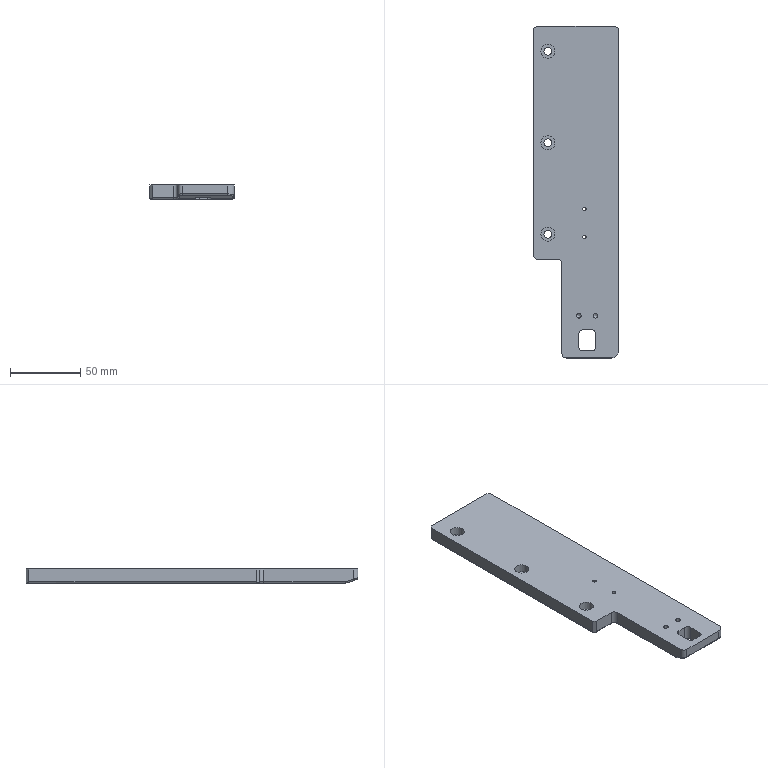NC program | NX | posted with a generic post | part box 60 x 236 x 10 mm
Lines 1 to 1176 of 2922:
N10 G17 G21 G94 G90
(FLOOR_WALL , TOOL : D80)
N12 T19 M6
N14 G54
N16 G17 G0 G90 X281. Y-30. S6500 M3
N18 G43 Z30. H19
N20 Z3.
N22 G94 G1 Z0. F1500.
N24 X278.
N26 X-42.
N28 X-45.
N30 Z3.
N32 G0 Z30.
N34 M5
(DRILLING , TOOL : D6A45)
N36 T01 M6
N38 G54
N40 G17 G0 G90 X18. Y-10. S9500 M3
N42 G43 Z30. H1
N44 G94 G81 G98 Z-1.8 F250. R3.
N46 X83.
N48 X130. Y-36.
N50 X150.
N52 X148. Y-10.
N54 G80
N56 G0 X148. Y-10. Z30.
N58 M5
(DRILLING_COPY_COPY , TOOL : 5.5ZT)
N60 T09 M6
N62 G54
N64 G17 G0 G90 X18. Y-10. S2000 M3
N66 G43 Z30. H9
N68 G94 G83 G98 Z-12.152 F150. Q2. R3.
N70 X83.
N72 X148.
N74 G80
N76 G0 X148. Y-10. Z30.
N78 M5
(DRILLING_COPY_COPY_COPY , TOOL : 2.5ZT)
N80 T02 M6
N82 G54
N84 G17 G0 G90 X130. Y-36. S2000 M3
N86 G43 Z30. H2
N88 G94 G83 G98 Z-11.101 F100. Q2. R3.
N90 X150.
N92 G80
N94 G0 X150. Y-36. Z30.
N96 M5
(ZLEVEL_PROFILE , TOOL : D10)
N98 T15 M6
N100 G54
N102 G17 G0 G90 X163.825 Y9.935 S9500 M3
N104 G43 Z30. H15
N106 Z0.5
N108 G94 G1 Z-1. F1000.
N110 X163.436 Y8.478
N112 G3 X163.695 Y7.512 R1.
N114 G1 X167.606 Y3.606 F3000.
N116 X169.606 Y1.606
N118 G2 X171.1 Y-2. R5.1
N120 G1 Y-14.9
N122 X232.971
N124 G2 X237.356 Y-16.175 R8.333
N126 X240.785 Y-20.779 R7.942
N128 X241.1 Y-23.02 R8.212
N130 G1 Y-54.977
N132 G2 X240.184 Y-59.287 R11.247
N134 X237.644 Y-62.662 R12.774
N136 X234.723 Y-64.384 R11.855
N138 X230.988 Y-65.098 R10.499
N140 G1 X229.803 Y-65.097
N142 X227.433
N144 G3 X226.567 Y-65.597 R1.
N146 G1 X225.701 Y-67.098
N148 Z0.5
N150 G0 X229.287 Y-67.1 Z-0.5
N152 G1 Z-2. F1000.
N154 X230.127 Y-65.608
N156 G2 X230.988 Y-65.099 R1.
N158 G3 X234.765 Y-64.369 R10.736 F3000.
N160 X237.644 Y-62.662 R11.866
N162 X240.184 Y-59.287 R12.774
N164 X241.1 Y-54.977 R11.247
N166 G1 Y-23.02
N168 G3 X240.785 Y-20.779 R8.212
N170 X237.333 Y-16.161 R7.942
N172 X232.971 Y-14.9 R8.333
N174 G1 X171.1
N176 Y-2.
N178 G3 X169.606 Y1.606 R5.1
N180 G1 X167.607 Y3.606
N182 G2 X167.348 Y4.572 R1.
N184 G1 X167.796 Y6.244
N186 Z-0.5
N188 G0 Y6.242 Z-1.5
N190 G1 Z-3. F1000.
N192 X167.348 Y4.572
N194 G3 X167.607 Y3.606 R1.
N196 G1 X169.606 Y1.606 F3000.
N198 G2 X171.1 Y-2. R5.1
N200 G1 Y-14.9
N202 X233.
N204 G2 X241.1 Y-23. R8.1
N206 G1 Y-55.
N208 G2 X238.813 Y-61.401 R10.1
N210 G1 X238.743 Y-61.485
N212 G2 X237.237 Y-62.944 R10.1
N214 G1 X237.12 Y-63.035
N216 G2 X231. Y-65.1 R10.1
N218 G3 X230.134 Y-65.6 R1.
N220 G1 X229.268 Y-67.1
N222 Z-1.5
N224 G0 Z30.
N226 X163.826 Y9.935
N228 Z-0.5
N230 G1 Z-2. F1000.
N232 X163.436 Y8.478
N234 G3 X163.696 Y7.512 R1.
N236 G1 X167.602 Y3.611 F3000.
N238 G3 X168.568 Y3.353 R1.
N240 G1 X170.239 Y3.802
N242 Z-0.5
N244 G0 X167.917 Y6.122 Z-1.5
N246 G1 Z-3. F1000.
N248 X166.694 Y4.898
N250 G2 X167.152 Y4.009 R1.
N252 G1 X167.154 Y4.056 F3000.
N254 X163.696 Y7.512
N256 G2 X163.437 Y8.478 R1.
N258 G1 X163.827 Y9.935
N260 Z-1.5
N262 G0 X163.826 Y9.936 Z-2.5
N264 G1 Z-4. F1000.
N266 X163.437 Y8.478
N268 G3 X163.696 Y7.512 R1.
N270 G1 X167.602 Y3.61 F3000.
N272 G3 X168.568 Y3.352 R1.
N274 G1 X170.24 Y3.801
N276 Z-2.5
N278 G0 Y3.8 Z-3.5
N280 G1 Z-5. F1000.
N282 X168.569 Y3.352
N284 G2 X167.603 Y3.61 R1.
N286 G1 X163.696 Y7.513 F3000.
N288 G2 X163.437 Y8.478 R1.
N290 G1 X163.827 Y9.936
N292 Z-3.5
N294 G0 Z-4.5
N296 G1 Z-6. F1000.
N298 X163.437 Y8.479
N300 G3 X163.696 Y7.513 R1.
N302 G1 X167.603 Y3.61 F3000.
N304 G3 X168.569 Y3.351 R1.
N306 G1 X170.241 Y3.8
N308 Z-4.5
N310 G0 Z-5.5
N312 G1 Z-7. F1000.
N314 X168.569 Y3.351
N316 G2 X167.603 Y3.609 R1.
N318 G1 X163.696 Y7.513 F3000.
N320 G2 X163.437 Y8.479 R1.
N322 G1 X163.827 Y9.936
N324 Z-5.5
N326 G0 Y9.937 Z-6.5
N328 G1 Z-8. F1000.
N330 X163.437 Y8.479
N332 G3 X163.697 Y7.513 R1.
N334 G1 X167.604 Y3.609 F3000.
N336 G3 X168.57 Y3.35 R1.
N338 G1 X170.242 Y3.799
N340 Z-6.5
N342 G0 Z-7.5
N344 G1 Z-9. F1000.
N346 X168.57 Y3.35
N348 G2 X167.604 Y3.609 R1.
N350 G1 X163.697 Y7.513 F3000.
N352 G2 X163.438 Y8.479 R1.
N354 G1 X163.828 Y9.937
N356 Z-7.5
N358 G0 Z-8.5
N360 G1 Z-10. F1000.
N362 X163.438 Y8.479
N364 G3 X163.697 Y7.513 R1.
N366 G1 X167.604 Y3.608 F3000.
N368 G3 X168.57 Y3.35 R1.
N370 G1 X170.243 Y3.798
N372 Z-8.5
N374 G0 Z30.
N376 X167.796 Y6.244
N378 Z-2.5
N380 G1 Z-4. F1000.
N382 X167.348 Y4.572
N384 G3 X167.607 Y3.606 R1.
N386 G1 X169.606 Y1.606 F3000.
N388 G2 X171.1 Y-2. R5.1
N390 G1 Y-14.9
N392 X233.
N394 G2 X241.1 Y-23. R8.1
N396 G1 Y-55.
N398 G2 X240.405 Y-58.681 R10.1
N400 G1 X239.846 Y-59.874
N402 G2 X238.813 Y-61.401 R10.1
N404 G1 X238.743 Y-61.485
N406 G2 X237.217 Y-62.96 R10.1
N408 G1 X237.12 Y-63.035
N410 G2 X231. Y-65.1 R10.1
N412 G3 X230.134 Y-65.6 R1.
N414 G1 X229.268 Y-67.1
N416 Z-2.5
N418 G0 Z-3.5
N420 G1 Z-5. F1000.
N422 X230.134 Y-65.6
N424 G2 X231. Y-65.1 R1.
N426 G3 X237.12 Y-63.035 R10.1 F3000.
N428 G1 X237.217 Y-62.96
N430 G3 X238.743 Y-61.485 R10.1
N432 G1 X238.813 Y-61.401
N434 G3 X239.846 Y-59.874 R10.1
N436 G1 X240.405 Y-58.681
N438 G3 X241.1 Y-55. R10.1
N440 G1 Y-23.
N442 G3 X233. Y-14.9 R8.1
N444 G1 X171.1
N446 Y-2.
N448 G3 X169.606 Y1.606 R5.1
N450 G1 X167.607 Y3.606
N452 G2 X167.348 Y4.572 R1.
N454 G1 X167.796 Y6.244
N456 Z-3.5
N458 G0 Z-4.5
N460 G1 Z-6. F1000.
N462 X167.348 Y4.572
N464 G3 X167.607 Y3.606 R1.
N466 G1 X169.606 Y1.606 F3000.
N468 G2 X171.1 Y-2. R5.1
N470 G1 Y-14.9
N472 X233.
N474 G2 X241.1 Y-23. R8.1
N476 G1 Y-55.
N478 G2 X240.405 Y-58.681 R10.1
N480 G1 X239.846 Y-59.874
N482 G2 X238.813 Y-61.401 R10.1
N484 G1 X238.743 Y-61.485
N486 G2 X237.217 Y-62.96 R10.1
N488 G1 X237.12 Y-63.035
N490 G2 X231. Y-65.1 R10.1
N492 G3 X230.134 Y-65.6 R1.
N494 G1 X229.268 Y-67.1
N496 Z-4.5
N498 G0 Z-5.5
N500 G1 Z-7. F1000.
N502 X230.134 Y-65.6
N504 G2 X231. Y-65.1 R1.
N506 G3 X237.12 Y-63.035 R10.1 F3000.
N508 G1 X237.217 Y-62.96
N510 G3 X238.743 Y-61.485 R10.1
N512 G1 X238.813 Y-61.401
N514 G3 X239.846 Y-59.874 R10.1
N516 G1 X240.405 Y-58.681
N518 G3 X241.1 Y-55. R10.1
N520 G1 Y-23.
N522 G3 X233. Y-14.9 R8.1
N524 G1 X171.1
N526 Y-2.
N528 G3 X169.606 Y1.606 R5.1
N530 G1 X167.607 Y3.606
N532 G2 X167.348 Y4.572 R1.
N534 G1 X167.796 Y6.244
N536 Z-5.5
N538 G0 Z-6.5
N540 G1 Z-8. F1000.
N542 X167.348 Y4.572
N544 G3 X167.607 Y3.606 R1.
N546 G1 X169.606 Y1.606 F3000.
N548 G2 X171.1 Y-2. R5.1
N550 G1 Y-14.9
N552 X233.
N554 G2 X241.1 Y-23. R8.1
N556 G1 Y-55.
N558 G2 X240.405 Y-58.681 R10.1
N560 G1 X239.846 Y-59.874
N562 G2 X238.813 Y-61.401 R10.1
N564 G1 X238.743 Y-61.485
N566 G2 X237.217 Y-62.96 R10.1
N568 G1 X237.12 Y-63.035
N570 G2 X231. Y-65.1 R10.1
N572 G3 X230.134 Y-65.6 R1.
N574 G1 X229.268 Y-67.1
N576 Z-6.5
N578 G0 Z-7.5
N580 G1 Z-9. F1000.
N582 X230.134 Y-65.6
N584 G2 X231. Y-65.1 R1.
N586 G3 X237.12 Y-63.035 R10.1 F3000.
N588 G1 X237.217 Y-62.96
N590 G3 X238.743 Y-61.485 R10.1
N592 G1 X238.813 Y-61.401
N594 G3 X239.846 Y-59.874 R10.1
N596 G1 X240.405 Y-58.681
N598 G3 X241.1 Y-55. R10.1
N600 G1 Y-23.
N602 G3 X233. Y-14.9 R8.1
N604 G1 X171.1
N606 Y-2.
N608 G3 X169.606 Y1.606 R5.1
N610 G1 X167.607 Y3.606
N612 G2 X167.348 Y4.572 R1.
N614 G1 X167.796 Y6.244
N616 Z-7.5
N618 G0 Z-8.5
N620 G1 Z-10. F1000.
N622 X167.348 Y4.572
N624 G3 X167.607 Y3.606 R1.
N626 G1 X169.606 Y1.606 F3000.
N628 G2 X171.1 Y-2. R5.1
N630 G1 Y-14.9
N632 X233.
N634 G2 X241.1 Y-23. R8.1
N636 G1 Y-55.
N638 G2 X240.405 Y-58.681 R10.1
N640 G1 X239.846 Y-59.874
N642 G2 X238.813 Y-61.401 R10.1
N644 G1 X238.743 Y-61.485
N646 G2 X237.217 Y-62.96 R10.1
N648 G1 X237.12 Y-63.035
N650 G2 X231. Y-65.1 R10.1
N652 G3 X230.134 Y-65.6 R1.
N654 G1 X229.268 Y-67.1
N656 Z-8.5
N658 G0 Z30.
(ZLEVEL_PROFILE_COPY , TOOL : D10)
N660 X2.159 Y-69.926
N662 Z0.5
N664 G1 Z-1. F1000.
N666 X2.55 Y-68.465
N668 G3 X2.291 Y-67.499 R1.
N670 G1 X-1.206 Y-64.003 F3000.
N672 X-1.606 Y-63.606
N674 X-3.606 Y-61.606
N676 G2 X-5.071 Y-57.459 R5.1
N678 G1 X-5.096 Y-57.407
N680 X-5.1 Y-57.016
N682 Y-2.874
N684 X-5.109 Y-2.802
N686 X-5.04 Y-2.779
N688 G2 X-3.606 Y1.606 R5.1
N690 G1 X-1.628 Y3.585
N692 G3 X-1.369 Y4.551 R1.
N694 G1 X-1.816 Y6.221
N696 Z0.5
N698 G0 X-1.796 Y6.243 Z-0.5
N700 G1 Z-2. F1000.
N702 X-1.348 Y4.572
N704 G2 X-1.607 Y3.606 R1.
N706 G1 X-3.606 Y1.606 F3000.
N708 G3 X-5.04 Y-2.779 R5.1
N710 G1 X-5.109 Y-2.802
N712 X-5.1 Y-2.874
N714 Y-57.016
N716 X-5.096 Y-57.407
N718 X-5.071 Y-57.459
N720 G3 X-3.606 Y-61.606 R5.1
N722 G1 X-1.606 Y-63.606
N724 G2 X-1.347 Y-64.572 R1.
N726 G1 X-1.795 Y-66.242
N728 Z-0.5
N730 G0 Z30.
N732 X2.158 Y-69.926
N734 Z-0.5
N736 G1 Z-2. F1000.
N738 X2.55 Y-68.465
N740 G3 X2.291 Y-67.499 R1.
N742 G1 X-1.206 Y-64.003 F3000.
N744 X-1.575 Y-63.637
N746 G3 X-2.542 Y-63.383 R1.
N748 G1 X-4.205 Y-63.836
N750 Z-0.5
N752 G0 X-4.207 Y-63.834 Z-1.5
N754 G1 Z-3. F1000.
N756 X-2.544 Y-63.381
N758 G2 X-1.577 Y-63.635 R1.
N760 G1 X-1.207 Y-64.003 F3000.
N762 X2.291 Y-67.499
N764 G2 X2.55 Y-68.465 R1.
N766 G1 X2.158 Y-69.926
N768 Z-1.5
N770 G0 X2.159 Y-69.927 Z-2.5
N772 G1 Z-4. F1000.
N774 X2.55 Y-68.465
N776 G3 X2.291 Y-67.499 R1.
N778 G1 X-1.603 Y-63.61 F3000.
N780 G3 X-2.569 Y-63.351 R1.
N782 G1 X-4.241 Y-63.8
N784 Z-2.5
N786 G0 Z-3.5
N788 G1 Z-5. F1000.
N790 X-2.569 Y-63.351
N792 G2 X-1.603 Y-63.609 R1.
N794 G1 X2.29 Y-67.5 F3000.
N796 G2 X2.55 Y-68.465 R1.
N798 G1 X2.159 Y-69.927
N800 Z-3.5
N802 G0 X2.158 Z-4.5
N804 G1 Z-6. F1000.
N806 X2.55 Y-68.465
N808 G3 X2.29 Y-67.5 R1.
N810 G1 X-1.603 Y-63.609 F3000.
N812 G3 X-2.569 Y-63.351 R1.
N814 G1 X-4.241 Y-63.799
N816 Z-4.5
N818 G0 X-4.242 Z-5.5
N820 G1 Z-7. F1000.
N822 X-2.57 Y-63.35
N824 G2 X-1.604 Y-63.609 R1.
N826 G1 X2.29 Y-67.5 F3000.
N828 G2 X2.549 Y-68.466 R1.
N830 G1 X2.158 Y-69.928
N832 Z-5.5
N834 G0 Z-6.5
N836 G1 Z-8. F1000.
N838 X2.549 Y-68.466
N840 G3 X2.29 Y-67.5 R1.
N842 G1 X-1.604 Y-63.609 F3000.
N844 G3 X-2.57 Y-63.35 R1.
N846 G1 X-4.242 Y-63.799
N848 Z-6.5
N850 G0 X-4.243 Y-63.798 Z-7.5
N852 G1 Z-9. F1000.
N854 X-2.57 Y-63.35
N856 G2 X-1.604 Y-63.608 R1.
N858 G1 X2.29 Y-67.5 F3000.
N860 G2 X2.549 Y-68.466 R1.
N862 G1 X2.158 Y-69.928
N864 Z-7.5
N866 G0 Z-8.5
N868 G1 Z-10. F1000.
N870 X2.549 Y-68.466
N872 G3 X2.29 Y-67.5 R1.
N874 G1 X-1.605 Y-63.608 F3000.
N876 G3 X-2.571 Y-63.349 R1.
N878 G1 X-4.243 Y-63.798
N880 Z-8.5
N882 G0 Z30.
N884 X-4.192 Y3.849
N886 Z0.5
N888 G1 Z-1. F1000.
N890 X-2.529 Y3.396
N892 G3 X-1.562 Y3.65 R1.
N894 G1 X-1.206 Y4.003 F3000.
N896 X2.291 Y7.499
N898 G3 X2.55 Y8.465 R1.
N900 G1 X2.159 Y9.926
N902 Z0.5
N904 G0 Z-0.5
N906 G1 Z-2. F1000.
N908 X2.55 Y8.465
N910 G2 X2.291 Y7.499 R1.
N912 G1 X-1.001 Y4.209 F3000.
N914 X-1.05 Y4.168
N916 X-1.006 Y4.12
N918 G2 X-1.141 Y5.111 R1.
N920 G1 X0.094 Y8.131
N922 Z-0.5
N924 G0 X-3.406 Y4.635 Z-1.5
N926 G1 Z-3. F1000.
N928 X-2.001 Y4.013
N930 G3 X-1.006 Y4.12 R1.
N932 G1 X-1.051 Y4.167 F3000.
N934 X-1.001 Y4.209
N936 X2.291 Y7.499
N938 G3 X2.55 Y8.465 R1.
N940 G1 X2.159 Y9.926
N942 Z-1.5
N944 G0 Z30.
N946 X-1.795 Y-66.243
N948 Z-1.5
N950 G1 Z-3. F1000.
N952 X-1.347 Y-64.572
N954 G3 X-1.606 Y-63.606 R1.
N956 G1 X-3.606 Y-61.606 F3000.
N958 G2 X-5.071 Y-57.459 R5.1
N960 G1 X-5.097 Y-57.407
N962 X-5.1 Y-57.016
N964 Y-2.874
N966 X-5.109 Y-2.802
N968 X-5.04 Y-2.779
N970 G2 X-3.606 Y1.606 R5.1
N972 G1 X-1.607 Y3.606
N974 G3 X-1.348 Y4.572 R1.
N976 G1 X-1.796 Y6.243
N978 Z-1.5
N980 G0 Z-2.5
N982 G1 Z-4. F1000.
N984 X-1.348 Y4.572
N986 G2 X-1.607 Y3.606 R1.
N988 G1 X-3.606 Y1.606 F3000.
N990 G3 X-5.04 Y-2.779 R5.1
N992 G1 X-5.105
N994 X-5.1 Y-2.843
N996 Y-57.016
N998 X-5.097 Y-57.407
N1000 X-5.071 Y-57.459
N1002 G3 X-3.606 Y-61.606 R5.1
N1004 G1 X-1.606 Y-63.606
N1006 G2 X-1.347 Y-64.572 R1.
N1008 G1 X-1.795 Y-66.244
N1010 Z-2.5
N1012 G0 Z30.
N1014 X-3.406 Y4.635
N1016 Z-2.5
N1018 G1 Z-4. F1000.
N1020 X-2.001 Y4.013
N1022 G3 X-1.006 Y4.12 R1.
N1024 G1 X-1.051 Y4.167 F3000.
N1026 X-1.001 Y4.209
N1028 X2.291 Y7.499
N1030 G3 X2.55 Y8.465 R1.
N1032 G1 X2.159 Y9.927
N1034 Z-2.5
N1036 G0 X2.158 Z-3.5
N1038 G1 Z-5. F1000.
N1040 X2.55 Y8.465
N1042 G2 X2.29 Y7.5 R1.
N1044 G1 X-1.002 Y4.209 F3000.
N1046 X-1.051 Y4.167
N1048 X-1.006 Y4.12
N1050 G2 X-1.163 Y5.107 R1.
N1052 G1 X-0.065 Y7.973
N1054 Z-3.5
N1056 G0 Z30.
N1058 X-1.796 Y-66.244
N1060 Z-3.5
N1062 G1 Z-5. F1000.
N1064 X-1.348 Y-64.572
N1066 G3 X-1.607 Y-63.606 R1.
N1068 G1 X-3.606 Y-61.606 F3000.
N1070 G2 X-5.071 Y-57.459 R5.1
N1072 G1 X-5.097 Y-57.407
N1074 X-5.1 Y-57.016
N1076 Y-2.843
N1078 X-5.105 Y-2.779
N1080 X-5.04
N1082 G2 X-3.606 Y1.606 R5.1
N1084 G1 X-1.606 Y3.606
N1086 G3 X-1.347 Y4.572 R1.
N1088 G1 X-1.795 Y6.244
N1090 Z-3.5
N1092 G0 Z-4.5
N1094 G1 Z-6. F1000.
N1096 X-1.347 Y4.572
N1098 G2 X-1.606 Y3.606 R1.
N1100 G1 X-3.606 Y1.606 F3000.
N1102 G3 X-5.04 Y-2.779 R5.1
N1104 G1 X-5.105
N1106 X-5.1 Y-2.843
N1108 Y-57.016
N1110 X-5.097 Y-57.407
N1112 X-5.071 Y-57.459
N1114 G3 X-3.606 Y-61.606 R5.1
N1116 G1 X-1.606 Y-63.606
N1118 G2 X-1.347 Y-64.572 R1.
N1120 G1 X-1.795 Y-66.244
N1122 Z-4.5
N1124 G0 Z30.
N1126 X-3.406 Y4.635
N1128 Z-4.5
N1130 G1 Z-6. F1000.
N1132 X-2.001 Y4.013
N1134 G3 X-1.006 Y4.12 R1.
N1136 G1 X-1.051 Y4.167 F3000.
N1138 X-1.002 Y4.209
N1140 X2.29 Y7.5
N1142 G3 X2.549 Y8.466 R1.
N1144 G1 X2.158 Y9.927
N1146 Z-4.5
N1148 G0 Z-5.5
N1150 G1 Z-7. F1000.
N1152 X2.549 Y8.466
N1154 G2 X2.29 Y7.5 R1.
N1156 G1 X-1.002 Y4.209 F3000.
N1158 X-1.052 Y4.166
N1160 X-1.006 Y4.12
N1162 G2 X-1.178 Y5.105 R1.
N1164 G1 X-0.162 Y7.876
N1166 Z-5.5
N1168 G0 Z30.
N1170 X-1.795 Y-66.245
N1172 Z-5.5
N1174 G1 Z-7. F1000.
N1176 X-1.347 Y-64.572
N1178 G3 X-1.606 Y-63.606 R1.
N1180 G1 X-3.606 Y-61.606 F3000.
N1182 G2 X-5.071 Y-57.459 R5.1
N1184 G1 X-5.097 Y-57.407
N1186 X-5.1 Y-57.016
N1188 Y-2.843
N1190 X-5.105 Y-2.779
N1192 X-5.04
N1194 G2 X-3.606 Y1.606 R5.1
N1196 G1 X-1.606 Y3.606
N1198 G3 X-1.347 Y4.572 R1.
N1200 G1 X-1.795 Y6.244
N1202 Z-5.5
N1204 G0 Z-6.5
N1206 G1 Z-8. F1000.
N1208 X-1.347 Y4.572
N1210 G2 X-1.606 Y3.606 R1.
N1212 G1 X-3.606 Y1.606 F3000.
N1214 G3 X-5.04 Y-2.779 R5.1
N1216 G1 X-5.105
N1218 X-5.1 Y-2.843
N1220 Y-57.016
N1222 X-5.097 Y-57.407
N1224 X-5.071 Y-57.459
N1226 G3 X-3.606 Y-61.606 R5.1
N1228 G1 X-1.606 Y-63.606
N1230 G2 X-1.347 Y-64.572 R1.
N1232 G1 X-1.796 Y-66.245
N1234 Z-6.5
N1236 G0 Z30.
N1238 X-3.406 Y4.635
N1240 Z-6.5
N1242 G1 Z-8. F1000.
N1244 X-2.001 Y4.013
N1246 G3 X-1.006 Y4.12 R1.
N1248 G1 X-1.052 Y4.166 F3000.
N1250 X-1.003 Y4.208
N1252 X2.29 Y7.5
N1254 G3 X2.549 Y8.466 R1.
N1256 G1 X2.158 Y9.927
N1258 Z-6.5
N1260 G0 X2.157 Z-7.5
N1262 G1 Z-9. F1000.
N1264 X2.549 Y8.466
N1266 G2 X2.29 Y7.5 R1.
N1268 G1 X-1.009 Y4.202 F3000.
N1270 X-1.006 Y4.12
N1272 Z-7.5
N1274 G0 Z30.
N1276 X-1.796 Y-66.245
N1278 Z-7.5
N1280 G1 Z-9. F1000.
N1282 X-1.347 Y-64.572
N1284 G3 X-1.606 Y-63.606 R1.
N1286 G1 X-3.606 Y-61.606 F3000.
N1288 G2 X-5.071 Y-57.459 R5.1
N1290 G1 X-5.097 Y-57.407
N1292 X-5.1 Y-57.016
N1294 Y-2.843
N1296 X-5.105 Y-2.779
N1298 X-5.04
N1300 G2 X-3.606 Y1.606 R5.1
N1302 G1 X-1.607 Y3.606
N1304 G3 X-1.348 Y4.572 R1.
N1306 G1 X-1.796 Y6.243
N1308 Z-7.5
N1310 G0 X-1.795 Y6.244 Z-8.5
N1312 G1 Z-10. F1000.
N1314 X-1.347 Y4.572
N1316 G2 X-1.606 Y3.606 R1.
N1318 G1 X-3.606 Y1.606 F3000.
N1320 G3 X-5.04 Y-2.779 R5.1
N1322 G1 X-5.105
N1324 X-5.1 Y-2.843
N1326 Y-57.016
N1328 X-5.097 Y-57.407
N1330 X-5.071 Y-57.459
N1332 G3 X-3.606 Y-61.606 R5.1
N1334 G1 X-1.606 Y-63.607
N1336 G2 X-1.347 Y-64.573 R1.
N1338 G1 X-1.795 Y-66.245
N1340 Z-8.5
N1342 G0 Z30.
N1344 X-3.406 Y4.635
N1346 Z-8.5
N1348 G1 Z-10. F1000.
N1350 X-2.001 Y4.013
N1352 G3 X-1.006 Y4.12 R1.
N1354 G1 X-1.009 Y4.202 F3000.
N1356 X2.29 Y7.5
N1358 G3 X2.549 Y8.466 R1.
N1360 G1 X2.157 Y9.927
N1362 Z-8.5
N1364 G0 Z30.
N1366 M5
(FLOOR_WALL_1 , TOOL : D10JING)
N1368 T14 M6
N1370 G54
N1372 G17 G0 G90 X165.955 Y6.5 S9500 M3
N1374 G43 Z30. H14
N1376 Z-8.5
N1378 G94 G1 Z-10. F1250.
N1380 X165.812 Y5.966
N1382 G3 X166.071 Y5. R1.
N1384 G1 X171. Y0.071
N1386 Y-15.
N1388 X233.
N1390 G2 X241. Y-23. R8.
N1392 G1 Y-55.
N1394 G2 X231. Y-65. R10.
N1396 G3 X230.134 Y-65.5 R1.
N1398 G1 X229.557 Y-66.5
N1400 Z-8.5
N1402 G0 Z30.
N1404 X0.045
N1406 Z-8.5
N1408 G1 Z-10.
N1410 X0.188 Y-65.966
N1412 G3 X-0.071 Y-65. R1.
N1414 G1 X-5. Y-60.071
N1416 Y0.071
N1418 X-0.071 Y5.
N1420 G3 X0.188 Y5.966 R1.
N1422 G1 X0.045 Y6.5
N1424 Z-8.5
N1426 G0 Z30.
N1428 M5
(ZLEVEL_PROFILE_COPY_1 , TOOL : D6)
N1430 T12 M6
N1432 G54
N1434 G17 G0 G90 X170.2 Y-13.954 S9500 M3
N1436 G43 Z30. H12
N1438 Z0.324
N1440 G94 G1 Z-1.176 F1000.
N1442 X169.3 Y-14.474
N1444 G3 X169. Y-14.994 R0.6
N1446 G1 Y-17. F1800.
N1448 X171.006
N1450 G3 X171.526 Y-16.7 R0.6
N1452 G1 X172.046 Y-15.8
N1454 Z0.324
N1456 G0 X170.2 Y-13.954 Z-0.265
N1458 G1 Z-1.765 F1000.
N1460 X169.3 Y-14.474
N1462 G3 X169. Y-14.994 R0.6
N1464 G1 Y-17. F1800.
N1466 X171.006
N1468 G3 X171.526 Y-16.7 R0.6
N1470 G1 X172.046 Y-15.8
N1472 Z-0.265
N1474 G0 X170.2 Y-13.954 Z-0.853
N1476 G1 Z-2.353 F1000.
N1478 X169.3 Y-14.474
N1480 G3 X169. Y-14.994 R0.6
N1482 G1 Y-17. F1800.
N1484 X171.006
N1486 G3 X171.526 Y-16.7 R0.6
N1488 G1 X172.046 Y-15.8
N1490 Z-0.853
N1492 G0 X170.2 Y-13.954 Z-1.441
N1494 G1 Z-2.941 F1000.
N1496 X169.3 Y-14.474
N1498 G3 X169. Y-14.994 R0.6
N1500 G1 Y-17. F1800.
N1502 X171.006
N1504 G3 X171.526 Y-16.7 R0.6
N1506 G1 X172.046 Y-15.8
N1508 Z-1.441
N1510 G0 X170.2 Y-13.954 Z-2.029
N1512 G1 Z-3.529 F1000.
N1514 X169.3 Y-14.474
N1516 G3 X169. Y-14.994 R0.6
N1518 G1 Y-17. F1800.
N1520 X171.006
N1522 G3 X171.526 Y-16.7 R0.6
N1524 G1 X172.046 Y-15.8
N1526 Z-2.029
N1528 G0 X170.2 Y-13.954 Z-2.618
N1530 G1 Z-4.118 F1000.
N1532 X169.3 Y-14.474
N1534 G3 X169. Y-14.994 R0.6
N1536 G1 Y-17. F1800.
N1538 X171.006
N1540 G3 X171.526 Y-16.7 R0.6
N1542 G1 X172.046 Y-15.8
N1544 Z-2.618
N1546 G0 X170.2 Y-13.954 Z-3.206
N1548 G1 Z-4.706 F1000.
N1550 X169.3 Y-14.474
N1552 G3 X169. Y-14.994 R0.6
N1554 G1 Y-17. F1800.
N1556 X171.006
N1558 G3 X171.526 Y-16.7 R0.6
N1560 G1 X172.046 Y-15.8
N1562 Z-3.206
N1564 G0 X170.2 Y-13.954 Z-3.794
N1566 G1 Z-5.294 F1000.
N1568 X169.3 Y-14.474
N1570 G3 X169. Y-14.994 R0.6
N1572 G1 Y-17. F1800.
N1574 X171.006
N1576 G3 X171.526 Y-16.7 R0.6
N1578 G1 X172.046 Y-15.8
N1580 Z-3.794
N1582 G0 X170.2 Y-13.954 Z-4.382
N1584 G1 Z-5.882 F1000.
N1586 X169.3 Y-14.474
N1588 G3 X169. Y-14.994 R0.6
N1590 G1 Y-17. F1800.
N1592 X171.006
N1594 G3 X171.526 Y-16.7 R0.6
N1596 G1 X172.046 Y-15.8
N1598 Z-4.382
N1600 G0 X170.2 Y-13.954 Z-4.971
N1602 G1 Z-6.471 F1000.
N1604 X169.3 Y-14.474
N1606 G3 X169. Y-14.994 R0.6
N1608 G1 Y-17. F1800.
N1610 X171.006
N1612 G3 X171.526 Y-16.7 R0.6
N1614 G1 X172.046 Y-15.8
N1616 Z-4.971
N1618 G0 X170.2 Y-13.954 Z-5.559
N1620 G1 Z-7.059 F1000.
N1622 X169.3 Y-14.474
N1624 G3 X169. Y-14.994 R0.6
N1626 G1 Y-17. F1800.
N1628 X171.006
N1630 G3 X171.526 Y-16.7 R0.6
N1632 G1 X172.046 Y-15.8
N1634 Z-5.559
N1636 G0 X170.2 Y-13.954 Z-6.147
N1638 G1 Z-7.647 F1000.
N1640 X169.3 Y-14.474
N1642 G3 X169. Y-14.994 R0.6
N1644 G1 Y-17. F1800.
N1646 X171.006
N1648 G3 X171.526 Y-16.7 R0.6
N1650 G1 X172.046 Y-15.8
N1652 Z-6.147
N1654 G0 X170.2 Y-13.954 Z-6.735
N1656 G1 Z-8.235 F1000.
N1658 X169.3 Y-14.474
N1660 G3 X169. Y-14.994 R0.6
N1662 G1 Y-17. F1800.
N1664 X171.006
N1666 G3 X171.526 Y-16.7 R0.6
N1668 G1 X172.046 Y-15.8
N1670 Z-6.735
N1672 G0 X170.2 Y-13.954 Z-7.324
N1674 G1 Z-8.824 F1000.
N1676 X169.3 Y-14.474
N1678 G3 X169. Y-14.994 R0.6
N1680 G1 Y-17. F1800.
N1682 X171.006
N1684 G3 X171.526 Y-16.7 R0.6
N1686 G1 X172.046 Y-15.8
N1688 Z-7.324
N1690 G0 X170.2 Y-13.954 Z-7.912
N1692 G1 Z-9.412 F1000.
N1694 X169.3 Y-14.474
N1696 G3 X169. Y-14.994 R0.6
N1698 G1 Y-17. F1800.
N1700 X171.006
N1702 G3 X171.526 Y-16.7 R0.6
N1704 G1 X172.046 Y-15.8
N1706 Z-7.912
N1708 G0 X170.2 Y-13.954 Z-8.5
N1710 G1 Z-10. F1000.
N1712 X169.3 Y-14.474
N1714 G3 X169. Y-14.994 R0.6
N1716 G1 Y-17. F1800.
N1718 X171.006
N1720 G3 X171.526 Y-16.7 R0.6
N1722 G1 X172.046 Y-15.8
N1724 Z-8.5
N1726 G0 Z30.
(ZLEVEL_PROFILE_1 , TOOL : D6)
N1728 X228. Y-40.398
N1730 Z1.5
N1732 G1 Y-35.007 Z1.217 F1000.
N1734 X227.979 Y-35. Z1.216
N1736 X219.017 Z0.747
N1738 X219. Y-35.102 Z0.741
N1740 Y-40.898 Z0.437
N1742 X219.017 Y-41. Z0.432
N1744 X228. Z-0.039
N1746 Y-35.007 Z-0.353
N1748 X227.979 Y-35. Z-0.354
N1750 X223.509 Z-0.588
N1752 X219.017 F1500.
N1754 X219. Y-35.102
N1756 Y-40.898
N1758 X219.017 Y-41.
N1760 X228.
N1762 Y-35.007
N1764 X227.979 Y-35.
N1766 X223.509
N1768 X221.297 Z-0.632
N1770 X219.095 Y-35.013 Z-0.676
N1772 X219.021 Y-35.034 Z-0.677
N1774 X219. Y-35.102 Z-0.678
N1776 Y-40.898 Z-0.792
N1778 X219.021 Y-40.966 Z-0.793
N1780 X219.095 Y-40.987 Z-0.794
N1782 X221.296 Y-41. Z-0.838
N1784 X223.508 Z-0.882
N1786 X225.752 Z-0.927
N1788 X227.994 Y-40.994 Z-0.971
N1790 X228. Y-39.002 Z-1.01
N1792 Y-37.008 Z-1.049
N1794 X227.995 Y-35.014 Z-1.088
N1796 X225.753 Y-35. Z-1.132
N1798 X223.509 Z-1.176
N1800 X221.297 Z-1.221
N1802 X219.095 Y-35.013 Z-1.265
N1804 X219.021 Y-35.034 Z-1.266
N1806 X219. Y-35.102 Z-1.267
N1808 Y-40.898 Z-1.38
N1810 X219.021 Y-40.966 Z-1.381
N1812 X219.095 Y-40.987 Z-1.383
N1814 X221.296 Y-41. Z-1.427
N1816 X223.508 Z-1.471
N1818 X225.752 Z-1.515
N1820 X227.994 Y-40.994 Z-1.559
N1822 X228. Y-39.002 Z-1.598
N1824 Y-37.008 Z-1.637
N1826 X227.995 Y-35.014 Z-1.677
N1828 X225.753 Y-35. Z-1.721
N1830 X223.509 Z-1.765
N1832 X221.297 Z-1.809
N1834 X219.095 Y-35.013 Z-1.853
N1836 X219.021 Y-35.034 Z-1.854
N1838 X219. Y-35.102 Z-1.855
N1840 Y-40.898 Z-1.969
N1842 X219.021 Y-40.966 Z-1.97
N1844 X219.095 Y-40.987 Z-1.971
N1846 X221.296 Y-41. Z-2.015
N1848 X223.508 Z-2.059
N1850 X225.752 Z-2.103
N1852 X227.994 Y-40.994 Z-2.147
N1854 X228. Y-39.002 Z-2.186
N1856 Y-37.008 Z-2.226
N1858 X227.995 Y-35.014 Z-2.265
N1860 X225.753 Y-35. Z-2.309
N1862 X223.509 Z-2.353
N1864 X221.297 Z-2.397
N1866 X219.095 Y-35.013 Z-2.441
N1868 X219.021 Y-35.034 Z-2.442
N1870 X219. Y-35.102 Z-2.443
N1872 Y-40.898 Z-2.557
N1874 X219.021 Y-40.966 Z-2.558
N1876 X219.095 Y-40.987 Z-2.559
N1878 X221.296 Y-41. Z-2.603
N1880 X223.508 Z-2.647
N1882 X225.752 Z-2.691
N1884 X227.993 Y-40.993 Z-2.735
N1886 X228. Y-39.002 Z-2.775
N1888 Y-37.008 Z-2.814
N1890 X227.995 Y-35.014 Z-2.853
N1892 X225.753 Y-35. Z-2.897
N1894 X223.509 Z-2.941
N1896 X221.297 Z-2.985
N1898 X219.096 Y-35.013 Z-3.029
N1900 X219.021 Y-35.034 Z-3.03
N1902 X219. Y-35.102 Z-3.031
N1904 Y-40.898 Z-3.145
N1906 X219.021 Y-40.966 Z-3.146
N1908 X219.096 Y-40.987 Z-3.147
N1910 X221.296 Y-41. Z-3.191
N1912 X223.508 Z-3.235
N1914 X225.752 Z-3.28
N1916 X227.993 Y-40.993 Z-3.324
N1918 X228. Y-39.002 Z-3.363
N1920 Y-37.008 Z-3.402
N1922 X227.994 Y-35.014 Z-3.441
N1924 X225.753 Y-35. Z-3.485
N1926 X223.509 Z-3.529
N1928 X221.297 Z-3.574
N1930 X219.096 Y-35.013 Z-3.618
N1932 X219.021 Y-35.034 Z-3.619
N1934 X219. Y-35.102 Z-3.62
N1936 Y-40.898 Z-3.733
N1938 X219.021 Y-40.966 Z-3.734
N1940 X219.096 Y-40.987 Z-3.735
N1942 X221.296 Y-41. Z-3.78
N1944 X223.509 Z-3.824
N1946 X225.752 Z-3.868
N1948 X227.993 Y-40.993 Z-3.912
N1950 X228. Y-39.002 Z-3.951
N1952 Y-37.008 Z-3.99
N1954 X227.994 Y-35.015 Z-4.03
N1956 X225.753 Y-35. Z-4.074
N1958 X223.509 Z-4.118
N1960 X221.297 Z-4.162
N1962 X219.096 Y-35.013 Z-4.206
N1964 X219.021 Y-35.034 Z-4.207
N1966 X219. Y-35.102 Z-4.208
N1968 Y-40.898 Z-4.322
N1970 X219.021 Y-40.966 Z-4.323
N1972 X219.096 Y-40.987 Z-4.324
N1974 X221.296 Y-41. Z-4.368
N1976 X223.509 Z-4.412
N1978 X225.752 Z-4.456
N1980 X227.993 Y-40.993 Z-4.5
N1982 X228. Y-39.002 Z-4.539
N1984 Y-37.009 Z-4.579
N1986 X227.994 Y-35.015 Z-4.618
N1988 X225.753 Y-35. Z-4.662
N1990 X223.509 Z-4.706
N1992 X221.297 Z-4.75
N1994 X219.096 Y-35.013 Z-4.794
N1996 X219.021 Y-35.034 Z-4.795
N1998 X219. Y-35.102 Z-4.796
N2000 Y-40.898 Z-4.91
N2002 X219.021 Y-40.966 Z-4.911
N2004 X219.096 Y-40.987 Z-4.912
N2006 X221.296 Y-41. Z-4.956
N2008 X223.509 Z-5.
N2010 X225.752 Z-5.044
N2012 X227.993 Y-40.993 Z-5.088
N2014 X228. Y-39.002 Z-5.127
N2016 Y-37.009 Z-5.167
N2018 X227.994 Y-35.015 Z-5.206
N2020 X225.753 Y-35. Z-5.25
N2022 X223.509 Z-5.294
N2024 X221.297 Z-5.338
N2026 X219.096 Y-35.013 Z-5.382
N2028 X219.021 Y-35.034 Z-5.383
N2030 X219. Y-35.102 Z-5.384
N2032 Y-40.898 Z-5.498
N2034 X219.021 Y-40.966 Z-5.499
N2036 X219.096 Y-40.987 Z-5.5
N2038 X221.296 Y-41. Z-5.544
N2040 X223.509 Z-5.588
N2042 X225.752 Z-5.632
N2044 X227.993 Y-40.993 Z-5.677
N2046 X228. Y-39.002 Z-5.716
N2048 Y-37.009 Z-5.755
N2050 X227.994 Y-35.015 Z-5.794
N2052 X225.753 Y-35. Z-5.838
N2054 X223.509 Z-5.882
N2056 X221.297 Z-5.926
N2058 X219.096 Y-35.013 Z-5.971
N2060 X219.021 Y-35.035 Z-5.972
N2062 X219. Y-35.102 Z-5.973
N2064 Y-40.898 Z-6.086
N2066 X219.021 Y-40.966 Z-6.087
N2068 X219.096 Y-40.987 Z-6.088
N2070 X221.296 Y-41. Z-6.132
N2072 X223.509 Z-6.177
N2074 X225.752 Z-6.221
N2076 X227.993 Y-40.993 Z-6.265
N2078 X228. Y-39.002 Z-6.304
N2080 Y-37.009 Z-6.343
N2082 X227.994 Y-35.015 Z-6.382
N2084 X225.753 Y-35. Z-6.427
N2086 X223.509 Z-6.471
N2088 X221.297 Z-6.515
N2090 X219.096 Y-35.013 Z-6.559
N2092 X219.021 Y-35.035 Z-6.56
N2094 X219. Y-35.102 Z-6.561
N2096 Y-40.898 Z-6.675
N2098 X219.021 Y-40.966 Z-6.676
N2100 X219.096 Y-40.987 Z-6.677
N2102 X221.297 Y-41. Z-6.721
N2104 X223.509 Z-6.765
N2106 X225.752 Z-6.809
N2108 X227.993 Y-40.993 Z-6.853
N2110 X228. Y-39.002 Z-6.892
N2112 Y-37.009 Z-6.931
N2114 X227.994 Y-35.015 Z-6.971
N2116 X225.753 Y-35. Z-7.015
N2118 X223.509 Z-7.059
N2120 X221.297 Z-7.103
N2122 X219.096 Y-35.013 Z-7.147
N2124 X219.021 Y-35.035 Z-7.148
N2126 X219. Y-35.102 Z-7.149
N2128 Y-40.898 Z-7.263
N2130 X219.021 Y-40.966 Z-7.264
N2132 X219.096 Y-40.987 Z-7.265
N2134 X221.297 Y-41. Z-7.309
N2136 X223.509 Z-7.353
N2138 X225.752 Z-7.397
N2140 X227.993 Y-40.993 Z-7.441
N2142 X228. Y-39.002 Z-7.48
N2144 Y-37.009 Z-7.52
N2146 X227.994 Y-35.015 Z-7.559
N2148 X225.753 Y-35. Z-7.603
N2150 X223.509 Z-7.647
N2152 X221.297 Z-7.691
N2154 X219.096 Y-35.013 Z-7.735
N2156 X219.021 Y-35.035 Z-7.736
N2158 X219. Y-35.102 Z-7.737
N2160 Y-40.898 Z-7.851
N2162 X219.021 Y-40.966 Z-7.852
N2164 X219.096 Y-40.987 Z-7.853
N2166 X221.297 Y-41. Z-7.897
N2168 X223.509 Z-7.941
N2170 X225.752 Z-7.985
N2172 X227.993 Y-40.993 Z-8.029
N2174 X228. Y-39.002 Z-8.069
N2176 Y-37.009 Z-8.108
N2178 X227.994 Y-35.016 Z-8.147
N2180 X225.753 Y-35. Z-8.191
N2182 X223.509 Z-8.235
N2184 X221.297 Z-8.279
N2186 X219.096 Y-35.013 Z-8.323
N2188 X219.021 Y-35.035 Z-8.325
N2190 X219. Y-35.102 Z-8.326
N2192 Y-40.898 Z-8.439
N2194 X219.021 Y-40.965 Z-8.44
N2196 X219.096 Y-40.987 Z-8.441
N2198 X221.297 Y-41. Z-8.485
N2200 X223.509 Z-8.53
N2202 X225.752 Z-8.574
N2204 X227.993 Y-40.993 Z-8.618
N2206 X228. Y-39.003 Z-8.657
N2208 Y-37.01 Z-8.696
N2210 X227.994 Y-35.017 Z-8.735
N2212 X225.753 Y-35. Z-8.779
N2214 X223.509 Z-8.824
N2216 X221.297 Z-8.868
N2218 X219.096 Y-35.013 Z-8.912
N2220 X219.021 Y-35.035 Z-8.913
N2222 X219. Y-35.102 Z-8.914
N2224 Y-40.898 Z-9.028
N2226 X219.021 Y-40.965 Z-9.029
N2228 X219.096 Y-40.987 Z-9.03
N2230 X221.297 Y-41. Z-9.074
N2232 X223.509 Z-9.118
N2234 X225.752 Z-9.162
N2236 X227.993 Y-40.993 Z-9.206
N2238 X228. Y-39.003 Z-9.245
N2240 Y-37.01 Z-9.284
N2242 X227.994 Y-35.017 Z-9.324
N2244 X225.753 Y-35. Z-9.368
N2246 X223.509 Z-9.412
N2248 X221.296 Z-9.456
N2250 X219.093 Y-35.013 Z-9.5
N2252 X219.02 Y-35.034 Z-9.501
N2254 X219. Y-35.102 Z-9.502
N2256 Y-40.898 Z-9.616
N2258 X219.021 Y-40.966 Z-9.617
N2260 X219.093 Y-40.987 Z-9.618
N2262 X221.296 Y-41. Z-9.662
N2264 X223.509 Z-9.706
N2266 X225.748 Z-9.75
N2268 X227.984 Y-40.996 Z-9.794
N2270 X228. Y-39.005 Z-9.833
N2272 Y-37.01 Z-9.873
N2274 X227.994 Y-35.016 Z-9.912
N2276 X225.753 Y-35. Z-9.956
N2278 X223.509 Z-10.
N2280 X219.017
N2282 X219. Y-35.102
N2284 Y-40.898
N2286 X219.017 Y-41.
N2288 X227.984
N2290 X228. Y-40.935
N2292 Y-35.007
N2294 X227.976 Y-35.
N2296 X223.509
N2298 Z-8.5
N2300 G0 Z30.
N2302 M5